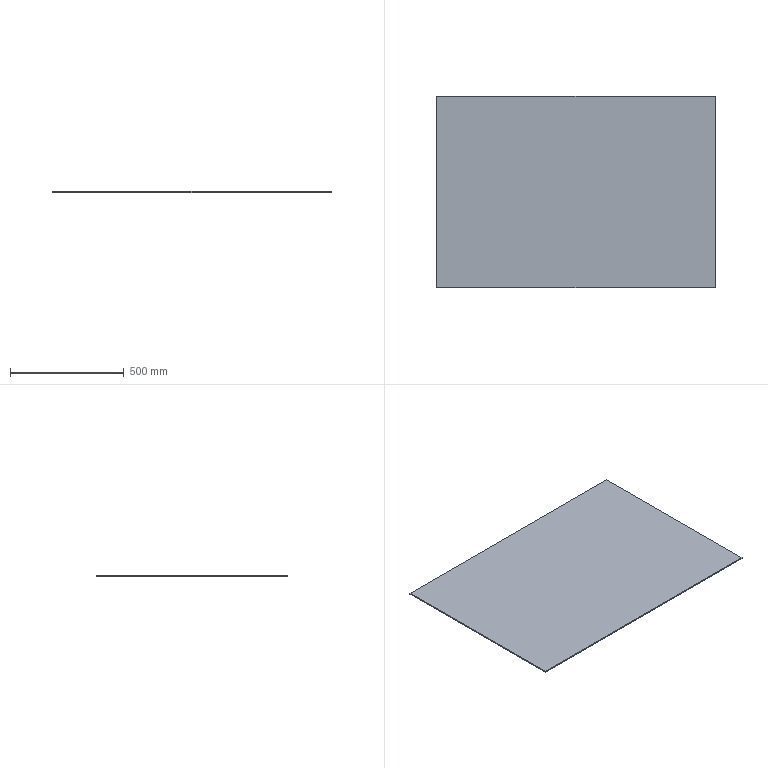Part | SolidWorks | features Extrusion 1, HoleWzd 1 | 1 solid | 6 faces | box 1226 x 842 x 5 mm | volume 5161460 mm3 | plane 6
STEP:
#1=CARTESIAN_POINT('',(613.,-421.,0.));
#2=VERTEX_POINT('',#1);
#3=CARTESIAN_POINT('',(613.,421.,0.));
#4=VERTEX_POINT('',#3);
#5=CARTESIAN_POINT('',(613.,421.,0.));
#6=DIRECTION('',(0.,1.,0.));
#7=VECTOR('',#6,1000.);
#8=LINE('',#5,#7);
#9=EDGE_CURVE('',#2,#4,#8,.T.);
#10=ORIENTED_EDGE('',*,*,#9,.T.);
#11=CARTESIAN_POINT('',(613.,421.,5.));
#12=VERTEX_POINT('',#11);
#13=CARTESIAN_POINT('',(613.,421.,5.));
#14=DIRECTION('',(0.,0.,-1.));
#15=VECTOR('',#14,1000.);
#16=LINE('',#13,#15);
#17=EDGE_CURVE('',#12,#4,#16,.T.);
#18=ORIENTED_EDGE('',*,*,#17,.F.);
#19=CARTESIAN_POINT('',(613.,-421.,5.));
#20=VERTEX_POINT('',#19);
#21=CARTESIAN_POINT('',(613.,421.,5.));
#22=DIRECTION('',(0.,1.,0.));
#23=VECTOR('',#22,1000.);
#24=LINE('',#21,#23);
#25=EDGE_CURVE('',#20,#12,#24,.T.);
#26=ORIENTED_EDGE('',*,*,#25,.F.);
#27=CARTESIAN_POINT('',(613.,-421.,5.));
#28=DIRECTION('',(0.,0.,-1.));
#29=VECTOR('',#28,1000.);
#30=LINE('',#27,#29);
#31=EDGE_CURVE('',#20,#2,#30,.T.);
#32=ORIENTED_EDGE('',*,*,#31,.T.);
#33=EDGE_LOOP('',(#10,#18,#26,#32));
#34=FACE_OUTER_BOUND('',#33,.T.);
#35=CARTESIAN_POINT('',(613.,421.,5.));
#36=DIRECTION('',(-1.,0.,0.));
#37=DIRECTION('',(0.,0.,1.));
#38=AXIS2_PLACEMENT_3D('',#35,#36,#37);
#39=PLANE('',#38);
#40=ADVANCED_FACE('',(#34),#39,.F.);
#41=CARTESIAN_POINT('',(-613.,421.,0.));
#42=VERTEX_POINT('',#41);
#43=CARTESIAN_POINT('',(-613.,421.,0.));
#44=DIRECTION('',(-1.,0.,0.));
#45=VECTOR('',#44,1000.);
#46=LINE('',#43,#45);
#47=EDGE_CURVE('',#4,#42,#46,.T.);
#48=ORIENTED_EDGE('',*,*,#47,.T.);
#49=CARTESIAN_POINT('',(-613.,421.,5.));
#50=VERTEX_POINT('',#49);
#51=CARTESIAN_POINT('',(-613.,421.,5.));
#52=DIRECTION('',(0.,0.,-1.));
#53=VECTOR('',#52,1000.);
#54=LINE('',#51,#53);
#55=EDGE_CURVE('',#50,#42,#54,.T.);
#56=ORIENTED_EDGE('',*,*,#55,.F.);
#57=CARTESIAN_POINT('',(-613.,421.,5.));
#58=DIRECTION('',(-1.,0.,0.));
#59=VECTOR('',#58,1000.);
#60=LINE('',#57,#59);
#61=EDGE_CURVE('',#12,#50,#60,.T.);
#62=ORIENTED_EDGE('',*,*,#61,.F.);
#63=ORIENTED_EDGE('',*,*,#17,.T.);
#64=EDGE_LOOP('',(#48,#56,#62,#63));
#65=FACE_OUTER_BOUND('',#64,.T.);
#66=CARTESIAN_POINT('',(-613.,421.,5.));
#67=DIRECTION('',(0.,-1.,0.));
#68=DIRECTION('',(0.,0.,-1.));
#69=AXIS2_PLACEMENT_3D('',#66,#67,#68);
#70=PLANE('',#69);
#71=ADVANCED_FACE('',(#65),#70,.F.);
#72=CARTESIAN_POINT('',(-613.,-421.,0.));
#73=VERTEX_POINT('',#72);
#74=CARTESIAN_POINT('',(-613.,421.,0.));
#75=DIRECTION('',(0.,-1.,0.));
#76=VECTOR('',#75,1000.);
#77=LINE('',#74,#76);
#78=EDGE_CURVE('',#42,#73,#77,.T.);
#79=ORIENTED_EDGE('',*,*,#78,.T.);
#80=CARTESIAN_POINT('',(-613.,-421.,5.));
#81=VERTEX_POINT('',#80);
#82=CARTESIAN_POINT('',(-613.,-421.,5.));
#83=DIRECTION('',(0.,0.,-1.));
#84=VECTOR('',#83,1000.);
#85=LINE('',#82,#84);
#86=EDGE_CURVE('',#81,#73,#85,.T.);
#87=ORIENTED_EDGE('',*,*,#86,.F.);
#88=CARTESIAN_POINT('',(-613.,421.,5.));
#89=DIRECTION('',(0.,-1.,0.));
#90=VECTOR('',#89,1000.);
#91=LINE('',#88,#90);
#92=EDGE_CURVE('',#50,#81,#91,.T.);
#93=ORIENTED_EDGE('',*,*,#92,.F.);
#94=ORIENTED_EDGE('',*,*,#55,.T.);
#95=EDGE_LOOP('',(#79,#87,#93,#94));
#96=FACE_OUTER_BOUND('',#95,.T.);
#97=CARTESIAN_POINT('',(-613.,421.,5.));
#98=DIRECTION('',(1.,0.,0.));
#99=DIRECTION('',(0.,0.,-1.));
#100=AXIS2_PLACEMENT_3D('',#97,#98,#99);
#101=PLANE('',#100);
#102=ADVANCED_FACE('',(#96),#101,.F.);
#103=CARTESIAN_POINT('',(-613.,-421.,0.));
#104=DIRECTION('',(1.,0.,0.));
#105=VECTOR('',#104,1000.);
#106=LINE('',#103,#105);
#107=EDGE_CURVE('',#73,#2,#106,.T.);
#108=ORIENTED_EDGE('',*,*,#107,.T.);
#109=ORIENTED_EDGE('',*,*,#31,.F.);
#110=CARTESIAN_POINT('',(-613.,-421.,5.));
#111=DIRECTION('',(1.,0.,0.));
#112=VECTOR('',#111,1000.);
#113=LINE('',#110,#112);
#114=EDGE_CURVE('',#81,#20,#113,.T.);
#115=ORIENTED_EDGE('',*,*,#114,.F.);
#116=ORIENTED_EDGE('',*,*,#86,.T.);
#117=EDGE_LOOP('',(#108,#109,#115,#116));
#118=FACE_OUTER_BOUND('',#117,.T.);
#119=CARTESIAN_POINT('',(-613.,-421.,5.));
#120=DIRECTION('',(0.,1.,0.));
#121=DIRECTION('',(0.,0.,1.));
#122=AXIS2_PLACEMENT_3D('',#119,#120,#121);
#123=PLANE('',#122);
#124=ADVANCED_FACE('',(#118),#123,.F.);
#125=ORIENTED_EDGE('',*,*,#25,.T.);
#126=ORIENTED_EDGE('',*,*,#61,.T.);
#127=ORIENTED_EDGE('',*,*,#92,.T.);
#128=ORIENTED_EDGE('',*,*,#114,.T.);
#129=EDGE_LOOP('',(#125,#126,#127,#128));
#130=FACE_OUTER_BOUND('',#129,.T.);
#131=CARTESIAN_POINT('',(0.,0.,5.));
#132=DIRECTION('',(0.,0.,1.));
#133=DIRECTION('',(1.,0.,0.));
#134=AXIS2_PLACEMENT_3D('',#131,#132,#133);
#135=PLANE('',#134);
#136=ADVANCED_FACE('',(#130),#135,.T.);
#137=ORIENTED_EDGE('',*,*,#9,.F.);
#138=ORIENTED_EDGE('',*,*,#107,.F.);
#139=ORIENTED_EDGE('',*,*,#78,.F.);
#140=ORIENTED_EDGE('',*,*,#47,.F.);
#141=EDGE_LOOP('',(#137,#138,#139,#140));
#142=FACE_OUTER_BOUND('',#141,.T.);
#143=CARTESIAN_POINT('',(0.,0.,0.));
#144=DIRECTION('',(0.,0.,1.));
#145=DIRECTION('',(1.,0.,0.));
#146=AXIS2_PLACEMENT_3D('',#143,#144,#145);
#147=PLANE('',#146);
#148=ADVANCED_FACE('',(#142),#147,.F.);
#149=CLOSED_SHELL('',(#40,#71,#102,#124,#136,#148));
#150=MANIFOLD_SOLID_BREP('',#149);
#151=CARTESIAN_POINT('',(0.,0.,0.));
#152=DIRECTION('',(0.,0.,1.));
#153=DIRECTION('',(1.,0.,0.));
#154=AXIS2_PLACEMENT_3D('',#151,#152,#153);
#155=(LENGTH_UNIT()NAMED_UNIT(*)SI_UNIT(.MILLI.,.METRE.));
#156=UNCERTAINTY_MEASURE_WITH_UNIT(LENGTH_MEASURE(0.00001),#155,'','');
#157=(NAMED_UNIT(*)PLANE_ANGLE_UNIT()SI_UNIT($,.RADIAN.));
#158=(NAMED_UNIT(*)SI_UNIT($,.STERADIAN.)SOLID_ANGLE_UNIT());
#159=(GEOMETRIC_REPRESENTATION_CONTEXT(3)GLOBAL_UNCERTAINTY_ASSIGNED_CONTEXT((#156))GLOBAL_UNIT_ASSIGNED_CONTEXT((#155,#157,#158))REPRESENTATION_CONTEXT('',''));
#160=ADVANCED_BREP_SHAPE_REPRESENTATION('',(#150,#154),#159);